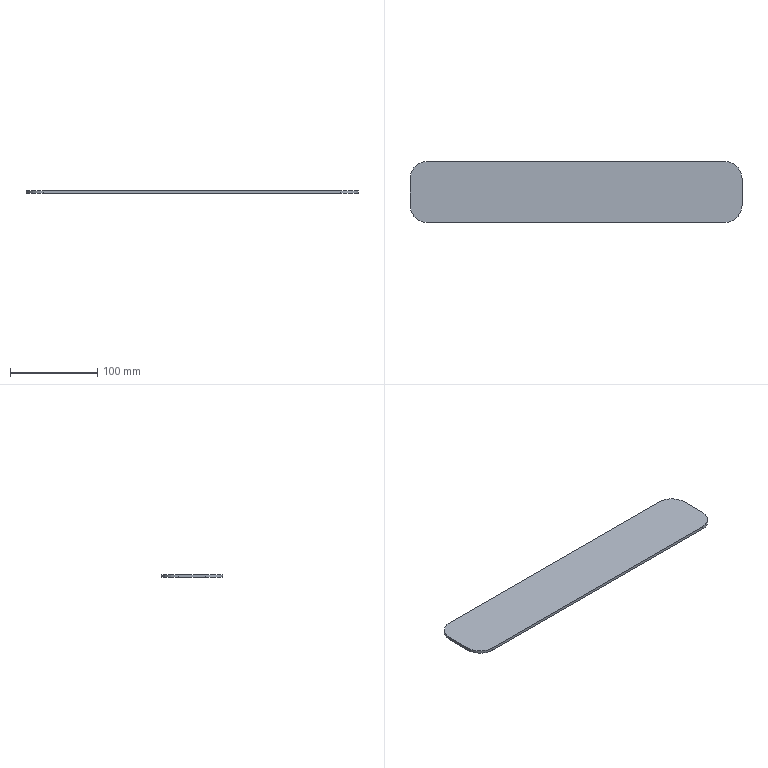Part | SolidWorks | features FlatPattern 1, SMBaseFlange 1, SheetMetal 1 | 1 solid | 10 faces | box 380 x 70 x 3.2 mm | volume 84021 mm3 | plane 6 | cylinder 4 | commonest cylinder face diameters 40 x4
STEP:
#1=CARTESIAN_POINT('',(225.291,52.617,0.));
#2=VERTEX_POINT('',#1);
#3=CARTESIAN_POINT('',(245.291,32.617,0.));
#4=VERTEX_POINT('',#3);
#5=CARTESIAN_POINT('',(225.291,32.617,0.));
#6=DIRECTION('',(0.,0.,-1.));
#7=DIRECTION('',(-1.,0.,0.));
#8=AXIS2_PLACEMENT_3D('',#5,#6,#7);
#9=CIRCLE('',#8,20.);
#10=EDGE_CURVE('',#2,#4,#9,.T.);
#11=ORIENTED_EDGE('',*,*,#10,.F.);
#12=CARTESIAN_POINT('',(225.291,52.617,3.2));
#13=VERTEX_POINT('',#12);
#14=CARTESIAN_POINT('',(225.291,52.617,3.2));
#15=DIRECTION('',(0.,0.,-1.));
#16=VECTOR('',#15,1000.);
#17=LINE('',#14,#16);
#18=EDGE_CURVE('',#13,#2,#17,.T.);
#19=ORIENTED_EDGE('',*,*,#18,.F.);
#20=CARTESIAN_POINT('',(245.291,32.617,3.2));
#21=VERTEX_POINT('',#20);
#22=CARTESIAN_POINT('',(225.291,32.617,3.2));
#23=DIRECTION('',(0.,0.,-1.));
#24=DIRECTION('',(-1.,0.,0.));
#25=AXIS2_PLACEMENT_3D('',#22,#23,#24);
#26=CIRCLE('',#25,20.);
#27=EDGE_CURVE('',#13,#21,#26,.T.);
#28=ORIENTED_EDGE('',*,*,#27,.T.);
#29=CARTESIAN_POINT('',(245.291,32.617,3.2));
#30=DIRECTION('',(0.,0.,-1.));
#31=VECTOR('',#30,1000.);
#32=LINE('',#29,#31);
#33=EDGE_CURVE('',#21,#4,#32,.T.);
#34=ORIENTED_EDGE('',*,*,#33,.T.);
#35=EDGE_LOOP('',(#11,#19,#28,#34));
#36=FACE_OUTER_BOUND('',#35,.T.);
#37=CARTESIAN_POINT('',(225.291,32.617,3.2));
#38=DIRECTION('',(0.,0.,-1.));
#39=DIRECTION('',(-1.,0.,0.));
#40=AXIS2_PLACEMENT_3D('',#37,#38,#39);
#41=CYLINDRICAL_SURFACE('',#40,20.);
#42=ADVANCED_FACE('',(#36),#41,.T.);
#43=CARTESIAN_POINT('',(-114.709,52.617,0.));
#44=VERTEX_POINT('',#43);
#45=CARTESIAN_POINT('',(-114.709,52.617,0.));
#46=DIRECTION('',(1.,0.,0.));
#47=VECTOR('',#46,1000.);
#48=LINE('',#45,#47);
#49=EDGE_CURVE('',#44,#2,#48,.T.);
#50=ORIENTED_EDGE('',*,*,#49,.F.);
#51=CARTESIAN_POINT('',(-114.709,52.617,3.2));
#52=VERTEX_POINT('',#51);
#53=CARTESIAN_POINT('',(-114.709,52.617,3.2));
#54=DIRECTION('',(0.,0.,-1.));
#55=VECTOR('',#54,1000.);
#56=LINE('',#53,#55);
#57=EDGE_CURVE('',#52,#44,#56,.T.);
#58=ORIENTED_EDGE('',*,*,#57,.F.);
#59=CARTESIAN_POINT('',(-114.709,52.617,3.2));
#60=DIRECTION('',(1.,0.,0.));
#61=VECTOR('',#60,1000.);
#62=LINE('',#59,#61);
#63=EDGE_CURVE('',#52,#13,#62,.T.);
#64=ORIENTED_EDGE('',*,*,#63,.T.);
#65=ORIENTED_EDGE('',*,*,#18,.T.);
#66=EDGE_LOOP('',(#50,#58,#64,#65));
#67=FACE_OUTER_BOUND('',#66,.T.);
#68=CARTESIAN_POINT('',(-114.709,52.617,3.2));
#69=DIRECTION('',(0.,1.,0.));
#70=DIRECTION('',(0.,0.,1.));
#71=AXIS2_PLACEMENT_3D('',#68,#69,#70);
#72=PLANE('',#71);
#73=ADVANCED_FACE('',(#67),#72,.T.);
#74=CARTESIAN_POINT('',(-134.709,32.617,0.));
#75=VERTEX_POINT('',#74);
#76=CARTESIAN_POINT('',(-114.709,32.617,0.));
#77=DIRECTION('',(0.,0.,-1.));
#78=DIRECTION('',(-1.,0.,0.));
#79=AXIS2_PLACEMENT_3D('',#76,#77,#78);
#80=CIRCLE('',#79,20.);
#81=EDGE_CURVE('',#75,#44,#80,.T.);
#82=ORIENTED_EDGE('',*,*,#81,.F.);
#83=CARTESIAN_POINT('',(-134.709,32.617,3.2));
#84=VERTEX_POINT('',#83);
#85=CARTESIAN_POINT('',(-134.709,32.617,3.2));
#86=DIRECTION('',(0.,0.,-1.));
#87=VECTOR('',#86,1000.);
#88=LINE('',#85,#87);
#89=EDGE_CURVE('',#84,#75,#88,.T.);
#90=ORIENTED_EDGE('',*,*,#89,.F.);
#91=CARTESIAN_POINT('',(-114.709,32.617,3.2));
#92=DIRECTION('',(0.,0.,-1.));
#93=DIRECTION('',(-1.,0.,0.));
#94=AXIS2_PLACEMENT_3D('',#91,#92,#93);
#95=CIRCLE('',#94,20.);
#96=EDGE_CURVE('',#84,#52,#95,.T.);
#97=ORIENTED_EDGE('',*,*,#96,.T.);
#98=ORIENTED_EDGE('',*,*,#57,.T.);
#99=EDGE_LOOP('',(#82,#90,#97,#98));
#100=FACE_OUTER_BOUND('',#99,.T.);
#101=CARTESIAN_POINT('',(-114.709,32.617,3.2));
#102=DIRECTION('',(0.,0.,-1.));
#103=DIRECTION('',(-1.,0.,0.));
#104=AXIS2_PLACEMENT_3D('',#101,#102,#103);
#105=CYLINDRICAL_SURFACE('',#104,20.);
#106=ADVANCED_FACE('',(#100),#105,.T.);
#107=CARTESIAN_POINT('',(-134.709,2.617,0.));
#108=VERTEX_POINT('',#107);
#109=CARTESIAN_POINT('',(-134.709,2.617,0.));
#110=DIRECTION('',(0.,1.,0.));
#111=VECTOR('',#110,1000.);
#112=LINE('',#109,#111);
#113=EDGE_CURVE('',#108,#75,#112,.T.);
#114=ORIENTED_EDGE('',*,*,#113,.F.);
#115=CARTESIAN_POINT('',(-134.709,2.617,3.2));
#116=VERTEX_POINT('',#115);
#117=CARTESIAN_POINT('',(-134.709,2.617,3.2));
#118=DIRECTION('',(0.,0.,-1.));
#119=VECTOR('',#118,1000.);
#120=LINE('',#117,#119);
#121=EDGE_CURVE('',#116,#108,#120,.T.);
#122=ORIENTED_EDGE('',*,*,#121,.F.);
#123=CARTESIAN_POINT('',(-134.709,2.617,3.2));
#124=DIRECTION('',(0.,1.,0.));
#125=VECTOR('',#124,1000.);
#126=LINE('',#123,#125);
#127=EDGE_CURVE('',#116,#84,#126,.T.);
#128=ORIENTED_EDGE('',*,*,#127,.T.);
#129=ORIENTED_EDGE('',*,*,#89,.T.);
#130=EDGE_LOOP('',(#114,#122,#128,#129));
#131=FACE_OUTER_BOUND('',#130,.T.);
#132=CARTESIAN_POINT('',(-134.709,2.617,3.2));
#133=DIRECTION('',(-1.,0.,0.));
#134=DIRECTION('',(0.,0.,1.));
#135=AXIS2_PLACEMENT_3D('',#132,#133,#134);
#136=PLANE('',#135);
#137=ADVANCED_FACE('',(#131),#136,.T.);
#138=CARTESIAN_POINT('',(-114.709,-17.383,0.));
#139=VERTEX_POINT('',#138);
#140=CARTESIAN_POINT('',(-114.709,2.617,0.));
#141=DIRECTION('',(0.,0.,-1.));
#142=DIRECTION('',(-1.,0.,0.));
#143=AXIS2_PLACEMENT_3D('',#140,#141,#142);
#144=CIRCLE('',#143,20.);
#145=EDGE_CURVE('',#139,#108,#144,.T.);
#146=ORIENTED_EDGE('',*,*,#145,.F.);
#147=CARTESIAN_POINT('',(-114.709,-17.383,3.2));
#148=VERTEX_POINT('',#147);
#149=CARTESIAN_POINT('',(-114.709,-17.383,3.2));
#150=DIRECTION('',(0.,0.,-1.));
#151=VECTOR('',#150,1000.);
#152=LINE('',#149,#151);
#153=EDGE_CURVE('',#148,#139,#152,.T.);
#154=ORIENTED_EDGE('',*,*,#153,.F.);
#155=CARTESIAN_POINT('',(-114.709,2.617,3.2));
#156=DIRECTION('',(0.,0.,-1.));
#157=DIRECTION('',(-1.,0.,0.));
#158=AXIS2_PLACEMENT_3D('',#155,#156,#157);
#159=CIRCLE('',#158,20.);
#160=EDGE_CURVE('',#148,#116,#159,.T.);
#161=ORIENTED_EDGE('',*,*,#160,.T.);
#162=ORIENTED_EDGE('',*,*,#121,.T.);
#163=EDGE_LOOP('',(#146,#154,#161,#162));
#164=FACE_OUTER_BOUND('',#163,.T.);
#165=CARTESIAN_POINT('',(-114.709,2.617,3.2));
#166=DIRECTION('',(0.,0.,-1.));
#167=DIRECTION('',(-1.,0.,0.));
#168=AXIS2_PLACEMENT_3D('',#165,#166,#167);
#169=CYLINDRICAL_SURFACE('',#168,20.);
#170=ADVANCED_FACE('',(#164),#169,.T.);
#171=CARTESIAN_POINT('',(225.291,-17.383,0.));
#172=VERTEX_POINT('',#171);
#173=CARTESIAN_POINT('',(225.291,-17.383,0.));
#174=DIRECTION('',(-1.,0.,0.));
#175=VECTOR('',#174,1000.);
#176=LINE('',#173,#175);
#177=EDGE_CURVE('',#172,#139,#176,.T.);
#178=ORIENTED_EDGE('',*,*,#177,.F.);
#179=CARTESIAN_POINT('',(225.291,-17.383,3.2));
#180=VERTEX_POINT('',#179);
#181=CARTESIAN_POINT('',(225.291,-17.383,3.2));
#182=DIRECTION('',(0.,0.,-1.));
#183=VECTOR('',#182,1000.);
#184=LINE('',#181,#183);
#185=EDGE_CURVE('',#180,#172,#184,.T.);
#186=ORIENTED_EDGE('',*,*,#185,.F.);
#187=CARTESIAN_POINT('',(225.291,-17.383,3.2));
#188=DIRECTION('',(-1.,0.,0.));
#189=VECTOR('',#188,1000.);
#190=LINE('',#187,#189);
#191=EDGE_CURVE('',#180,#148,#190,.T.);
#192=ORIENTED_EDGE('',*,*,#191,.T.);
#193=ORIENTED_EDGE('',*,*,#153,.T.);
#194=EDGE_LOOP('',(#178,#186,#192,#193));
#195=FACE_OUTER_BOUND('',#194,.T.);
#196=CARTESIAN_POINT('',(225.291,-17.383,3.2));
#197=DIRECTION('',(0.,-1.,0.));
#198=DIRECTION('',(0.,0.,-1.));
#199=AXIS2_PLACEMENT_3D('',#196,#197,#198);
#200=PLANE('',#199);
#201=ADVANCED_FACE('',(#195),#200,.T.);
#202=CARTESIAN_POINT('',(245.291,2.617,0.));
#203=VERTEX_POINT('',#202);
#204=CARTESIAN_POINT('',(225.291,2.617,0.));
#205=DIRECTION('',(0.,0.,-1.));
#206=DIRECTION('',(-1.,0.,0.));
#207=AXIS2_PLACEMENT_3D('',#204,#205,#206);
#208=CIRCLE('',#207,20.);
#209=EDGE_CURVE('',#203,#172,#208,.T.);
#210=ORIENTED_EDGE('',*,*,#209,.F.);
#211=CARTESIAN_POINT('',(245.291,2.617,3.2));
#212=VERTEX_POINT('',#211);
#213=CARTESIAN_POINT('',(245.291,2.617,3.2));
#214=DIRECTION('',(0.,0.,-1.));
#215=VECTOR('',#214,1000.);
#216=LINE('',#213,#215);
#217=EDGE_CURVE('',#212,#203,#216,.T.);
#218=ORIENTED_EDGE('',*,*,#217,.F.);
#219=CARTESIAN_POINT('',(225.291,2.617,3.2));
#220=DIRECTION('',(0.,0.,-1.));
#221=DIRECTION('',(-1.,0.,0.));
#222=AXIS2_PLACEMENT_3D('',#219,#220,#221);
#223=CIRCLE('',#222,20.);
#224=EDGE_CURVE('',#212,#180,#223,.T.);
#225=ORIENTED_EDGE('',*,*,#224,.T.);
#226=ORIENTED_EDGE('',*,*,#185,.T.);
#227=EDGE_LOOP('',(#210,#218,#225,#226));
#228=FACE_OUTER_BOUND('',#227,.T.);
#229=CARTESIAN_POINT('',(225.291,2.617,3.2));
#230=DIRECTION('',(0.,0.,-1.));
#231=DIRECTION('',(-1.,0.,0.));
#232=AXIS2_PLACEMENT_3D('',#229,#230,#231);
#233=CYLINDRICAL_SURFACE('',#232,20.);
#234=ADVANCED_FACE('',(#228),#233,.T.);
#235=CARTESIAN_POINT('',(245.291,32.617,0.));
#236=DIRECTION('',(0.,-1.,0.));
#237=VECTOR('',#236,1000.);
#238=LINE('',#235,#237);
#239=EDGE_CURVE('',#4,#203,#238,.T.);
#240=ORIENTED_EDGE('',*,*,#239,.F.);
#241=ORIENTED_EDGE('',*,*,#33,.F.);
#242=CARTESIAN_POINT('',(245.291,32.617,3.2));
#243=DIRECTION('',(0.,-1.,0.));
#244=VECTOR('',#243,1000.);
#245=LINE('',#242,#244);
#246=EDGE_CURVE('',#21,#212,#245,.T.);
#247=ORIENTED_EDGE('',*,*,#246,.T.);
#248=ORIENTED_EDGE('',*,*,#217,.T.);
#249=EDGE_LOOP('',(#240,#241,#247,#248));
#250=FACE_OUTER_BOUND('',#249,.T.);
#251=CARTESIAN_POINT('',(245.291,32.617,3.2));
#252=DIRECTION('',(1.,0.,0.));
#253=DIRECTION('',(0.,0.,-1.));
#254=AXIS2_PLACEMENT_3D('',#251,#252,#253);
#255=PLANE('',#254);
#256=ADVANCED_FACE('',(#250),#255,.T.);
#257=ORIENTED_EDGE('',*,*,#27,.F.);
#258=ORIENTED_EDGE('',*,*,#63,.F.);
#259=ORIENTED_EDGE('',*,*,#96,.F.);
#260=ORIENTED_EDGE('',*,*,#127,.F.);
#261=ORIENTED_EDGE('',*,*,#160,.F.);
#262=ORIENTED_EDGE('',*,*,#191,.F.);
#263=ORIENTED_EDGE('',*,*,#224,.F.);
#264=ORIENTED_EDGE('',*,*,#246,.F.);
#265=EDGE_LOOP('',(#257,#258,#259,#260,#261,#262,#263,#264));
#266=FACE_OUTER_BOUND('',#265,.T.);
#267=CARTESIAN_POINT('',(225.291,32.617,3.2));
#268=DIRECTION('',(0.,0.,-1.));
#269=DIRECTION('',(-1.,0.,0.));
#270=AXIS2_PLACEMENT_3D('',#267,#268,#269);
#271=PLANE('',#270);
#272=ADVANCED_FACE('',(#266),#271,.F.);
#273=ORIENTED_EDGE('',*,*,#10,.T.);
#274=ORIENTED_EDGE('',*,*,#239,.T.);
#275=ORIENTED_EDGE('',*,*,#209,.T.);
#276=ORIENTED_EDGE('',*,*,#177,.T.);
#277=ORIENTED_EDGE('',*,*,#145,.T.);
#278=ORIENTED_EDGE('',*,*,#113,.T.);
#279=ORIENTED_EDGE('',*,*,#81,.T.);
#280=ORIENTED_EDGE('',*,*,#49,.T.);
#281=EDGE_LOOP('',(#273,#274,#275,#276,#277,#278,#279,#280));
#282=FACE_OUTER_BOUND('',#281,.T.);
#283=CARTESIAN_POINT('',(225.291,32.617,0.));
#284=DIRECTION('',(0.,0.,-1.));
#285=DIRECTION('',(-1.,0.,0.));
#286=AXIS2_PLACEMENT_3D('',#283,#284,#285);
#287=PLANE('',#286);
#288=ADVANCED_FACE('',(#282),#287,.T.);
#289=CLOSED_SHELL('',(#42,#73,#106,#137,#170,#201,#234,#256,#272,#288));
#290=MANIFOLD_SOLID_BREP('',#289);
#291=CARTESIAN_POINT('',(0.,0.,0.));
#292=DIRECTION('',(0.,0.,1.));
#293=DIRECTION('',(1.,0.,0.));
#294=AXIS2_PLACEMENT_3D('',#291,#292,#293);
#295=(LENGTH_UNIT()NAMED_UNIT(*)SI_UNIT(.MILLI.,.METRE.));
#296=UNCERTAINTY_MEASURE_WITH_UNIT(LENGTH_MEASURE(0.00001),#295,'','');
#297=(NAMED_UNIT(*)PLANE_ANGLE_UNIT()SI_UNIT($,.RADIAN.));
#298=(NAMED_UNIT(*)SI_UNIT($,.STERADIAN.)SOLID_ANGLE_UNIT());
#299=(GEOMETRIC_REPRESENTATION_CONTEXT(3)GLOBAL_UNCERTAINTY_ASSIGNED_CONTEXT((#296))GLOBAL_UNIT_ASSIGNED_CONTEXT((#295,#297,#298))REPRESENTATION_CONTEXT('',''));
#300=ADVANCED_BREP_SHAPE_REPRESENTATION('',(#290,#294),#299);